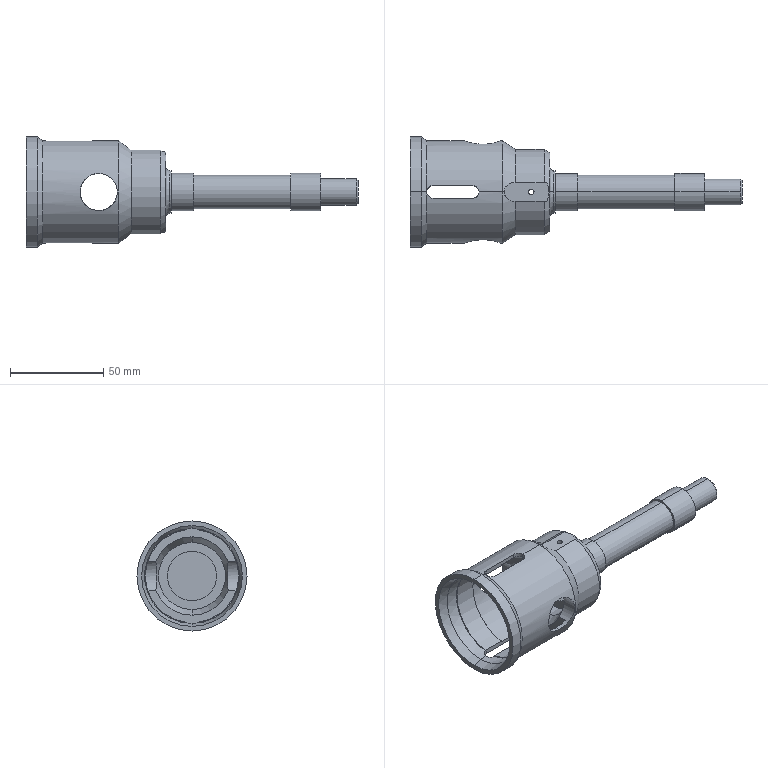Part | SolidWorks | features ICE 3, MirrorPattern 1, Revolution 1 | 1 solid | 82 faces | box 178 x 59 x 59 mm | volume 74305 mm3 | cylinder 43 | plane 25 | cone 12 | torus 2 | commonest cylinder face diameters 20 x8 7 x6 3 x4 51 x4 10 x3 14 x2